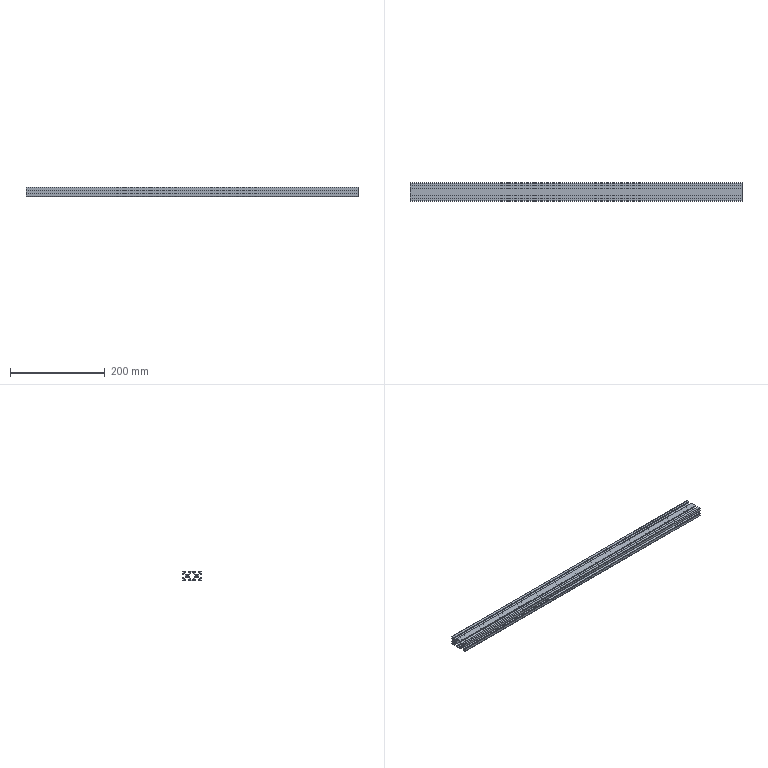Part | NX | features DATUM_CSYS 2, EXTRUDE 1, SKETCH 1 | 1 solid | 108 faces | box 700 x 40 x 20 mm | volume 206899 mm3 | plane 102 | cylinder 6 | commonest cylinder face diameters 3 x4 5 x2